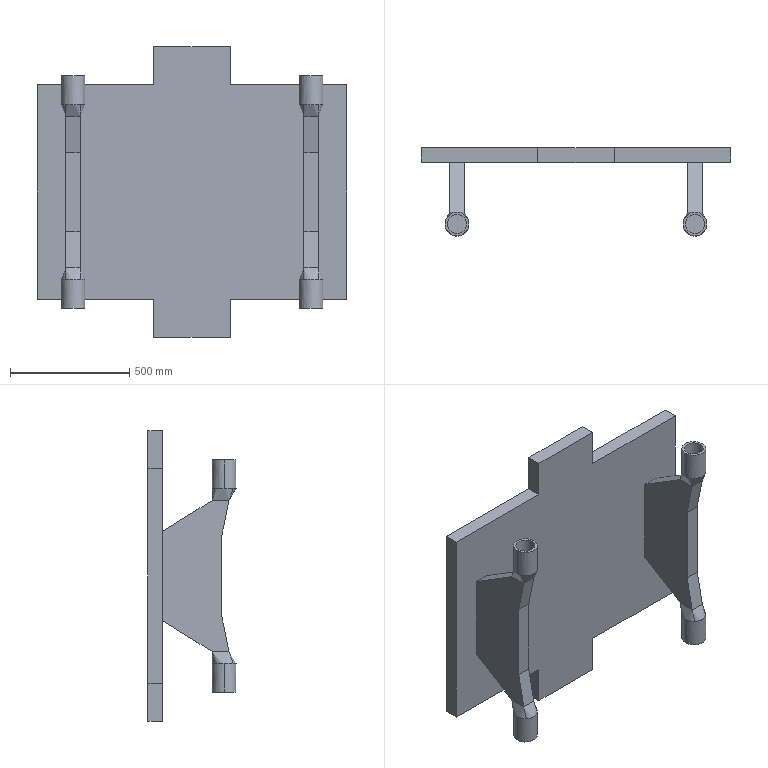Part | SolidWorks | features ICE 3, MirrorSolid 2, Blend 1, Extrusion 1, LPattern 1, MirrorPattern 1, RefPoint 1 | 6 solids | 90 faces | box 1300 x 370 x 1220 mm | volume 96223976 mm3 | plane 46 | cylinder 28 | spline 16 | commonest cylinder face diameters 80 x14 100 x14